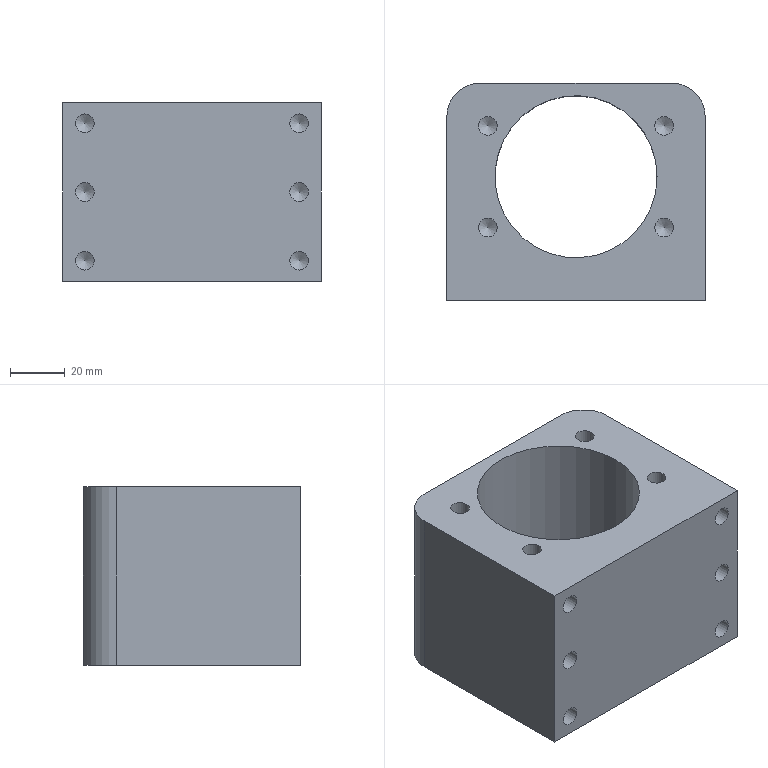Part | NX | 1 solid | 29 faces | box 94 x 79 x 65 mm | volume 292691 mm3 | cylinder 13 | cone 10 | plane 6 | commonest cylinder face diameters 6.8 x10 24 x2 59 x1
STEP:
#1=CARTESIAN_POINT('',(47.,-39.5,0.));
#2=VERTEX_POINT('',#1);
#3=CARTESIAN_POINT('',(47.,27.5,0.));
#4=VERTEX_POINT('',#3);
#5=CARTESIAN_POINT('',(47.,39.5,0.));
#6=DIRECTION('',(0.,1.,0.));
#7=VECTOR('',#6,1000.);
#8=LINE('',#5,#7);
#9=EDGE_CURVE('',#2,#4,#8,.T.);
#10=ORIENTED_EDGE('',*,*,#9,.T.);
#11=CARTESIAN_POINT('',(47.,27.5,65.));
#12=VERTEX_POINT('',#11);
#13=CARTESIAN_POINT('',(47.,27.5,65.));
#14=DIRECTION('',(0.,0.,-1.));
#15=VECTOR('',#14,1000.);
#16=LINE('',#13,#15);
#17=EDGE_CURVE('',#4,#12,#16,.F.);
#18=ORIENTED_EDGE('',*,*,#17,.T.);
#19=CARTESIAN_POINT('',(47.,-39.5,65.));
#20=VERTEX_POINT('',#19);
#21=CARTESIAN_POINT('',(47.,39.5,65.));
#22=DIRECTION('',(0.,1.,0.));
#23=VECTOR('',#22,1000.);
#24=LINE('',#21,#23);
#25=EDGE_CURVE('',#20,#12,#24,.T.);
#26=ORIENTED_EDGE('',*,*,#25,.F.);
#27=CARTESIAN_POINT('',(47.,-39.5,65.));
#28=DIRECTION('',(0.,0.,-1.));
#29=VECTOR('',#28,1000.);
#30=LINE('',#27,#29);
#31=EDGE_CURVE('',#20,#2,#30,.T.);
#32=ORIENTED_EDGE('',*,*,#31,.T.);
#33=EDGE_LOOP('',(#10,#18,#26,#32));
#34=FACE_BOUND('',#33,.T.);
#35=CARTESIAN_POINT('',(47.,39.5,65.));
#36=DIRECTION('',(-1.,0.,0.));
#37=DIRECTION('',(0.,-1.,0.));
#38=AXIS2_PLACEMENT_3D('',#35,#36,#37);
#39=PLANE('',#38);
#40=ADVANCED_FACE('',(#34),#39,.F.);
#41=CARTESIAN_POINT('',(35.,39.5,0.));
#42=VERTEX_POINT('',#41);
#43=CARTESIAN_POINT('',(-35.,39.5,0.));
#44=VERTEX_POINT('',#43);
#45=CARTESIAN_POINT('',(-47.,39.5,0.));
#46=DIRECTION('',(-1.,0.,0.));
#47=VECTOR('',#46,1000.);
#48=LINE('',#45,#47);
#49=EDGE_CURVE('',#42,#44,#48,.T.);
#50=ORIENTED_EDGE('',*,*,#49,.T.);
#51=CARTESIAN_POINT('',(-35.,39.5,65.));
#52=VERTEX_POINT('',#51);
#53=CARTESIAN_POINT('',(-35.,39.5,65.));
#54=DIRECTION('',(0.,0.,-1.));
#55=VECTOR('',#54,1000.);
#56=LINE('',#53,#55);
#57=EDGE_CURVE('',#44,#52,#56,.F.);
#58=ORIENTED_EDGE('',*,*,#57,.T.);
#59=CARTESIAN_POINT('',(35.,39.5,65.));
#60=VERTEX_POINT('',#59);
#61=CARTESIAN_POINT('',(-47.,39.5,65.));
#62=DIRECTION('',(-1.,0.,0.));
#63=VECTOR('',#62,1000.);
#64=LINE('',#61,#63);
#65=EDGE_CURVE('',#60,#52,#64,.T.);
#66=ORIENTED_EDGE('',*,*,#65,.F.);
#67=CARTESIAN_POINT('',(35.,39.5,65.));
#68=DIRECTION('',(0.,0.,-1.));
#69=VECTOR('',#68,1000.);
#70=LINE('',#67,#69);
#71=EDGE_CURVE('',#60,#42,#70,.T.);
#72=ORIENTED_EDGE('',*,*,#71,.T.);
#73=EDGE_LOOP('',(#50,#58,#66,#72));
#74=FACE_BOUND('',#73,.T.);
#75=CARTESIAN_POINT('',(-47.,39.5,65.));
#76=DIRECTION('',(0.,-1.,0.));
#77=DIRECTION('',(0.,0.,-1.));
#78=AXIS2_PLACEMENT_3D('',#75,#76,#77);
#79=PLANE('',#78);
#80=ADVANCED_FACE('',(#74),#79,.F.);
#81=CARTESIAN_POINT('',(-47.,27.5,65.));
#82=VERTEX_POINT('',#81);
#83=CARTESIAN_POINT('',(-47.,-39.5,65.));
#84=VERTEX_POINT('',#83);
#85=CARTESIAN_POINT('',(-47.,39.5,65.));
#86=DIRECTION('',(0.,-1.,0.));
#87=VECTOR('',#86,1000.);
#88=LINE('',#85,#87);
#89=EDGE_CURVE('',#82,#84,#88,.T.);
#90=ORIENTED_EDGE('',*,*,#89,.F.);
#91=CARTESIAN_POINT('',(-47.,27.5,0.));
#92=VERTEX_POINT('',#91);
#93=CARTESIAN_POINT('',(-47.,27.5,65.));
#94=DIRECTION('',(0.,0.,-1.));
#95=VECTOR('',#94,1000.);
#96=LINE('',#93,#95);
#97=EDGE_CURVE('',#82,#92,#96,.T.);
#98=ORIENTED_EDGE('',*,*,#97,.T.);
#99=CARTESIAN_POINT('',(-47.,-39.5,0.));
#100=VERTEX_POINT('',#99);
#101=CARTESIAN_POINT('',(-47.,39.5,0.));
#102=DIRECTION('',(0.,-1.,0.));
#103=VECTOR('',#102,1000.);
#104=LINE('',#101,#103);
#105=EDGE_CURVE('',#92,#100,#104,.T.);
#106=ORIENTED_EDGE('',*,*,#105,.T.);
#107=CARTESIAN_POINT('',(-47.,-39.5,65.));
#108=DIRECTION('',(0.,0.,-1.));
#109=VECTOR('',#108,1000.);
#110=LINE('',#107,#109);
#111=EDGE_CURVE('',#84,#100,#110,.T.);
#112=ORIENTED_EDGE('',*,*,#111,.F.);
#113=EDGE_LOOP('',(#90,#98,#106,#112));
#114=FACE_BOUND('',#113,.T.);
#115=CARTESIAN_POINT('',(-47.,39.5,65.));
#116=DIRECTION('',(1.,0.,0.));
#117=DIRECTION('',(0.,1.,0.));
#118=AXIS2_PLACEMENT_3D('',#115,#116,#117);
#119=PLANE('',#118);
#120=ADVANCED_FACE('',(#114),#119,.F.);
#121=CARTESIAN_POINT('',(-39.,-39.5,54.1));
#122=VERTEX_POINT('',#121);
#123=CARTESIAN_POINT('',(-39.,-39.5,57.5));
#124=DIRECTION('',(0.,-1.,0.));
#125=DIRECTION('',(0.,0.,-1.));
#126=AXIS2_PLACEMENT_3D('',#123,#124,#125);
#127=CIRCLE('',#126,3.4);
#128=EDGE_CURVE('',#122,#122,#127,.T.);
#129=ORIENTED_EDGE('',*,*,#128,.F.);
#130=EDGE_LOOP('',(#129));
#131=FACE_BOUND('',#130,.T.);
#132=CARTESIAN_POINT('',(39.,-39.5,54.1));
#133=VERTEX_POINT('',#132);
#134=CARTESIAN_POINT('',(39.,-39.5,57.5));
#135=DIRECTION('',(0.,-1.,0.));
#136=DIRECTION('',(0.,0.,-1.));
#137=AXIS2_PLACEMENT_3D('',#134,#135,#136);
#138=CIRCLE('',#137,3.4);
#139=EDGE_CURVE('',#133,#133,#138,.T.);
#140=ORIENTED_EDGE('',*,*,#139,.F.);
#141=EDGE_LOOP('',(#140));
#142=FACE_BOUND('',#141,.T.);
#143=CARTESIAN_POINT('',(39.,-39.5,29.1));
#144=VERTEX_POINT('',#143);
#145=CARTESIAN_POINT('',(39.,-39.5,32.5));
#146=DIRECTION('',(0.,-1.,0.));
#147=DIRECTION('',(0.,0.,-1.));
#148=AXIS2_PLACEMENT_3D('',#145,#146,#147);
#149=CIRCLE('',#148,3.4);
#150=EDGE_CURVE('',#144,#144,#149,.T.);
#151=ORIENTED_EDGE('',*,*,#150,.F.);
#152=EDGE_LOOP('',(#151));
#153=FACE_BOUND('',#152,.T.);
#154=CARTESIAN_POINT('',(-39.,-39.5,29.1));
#155=VERTEX_POINT('',#154);
#156=CARTESIAN_POINT('',(-39.,-39.5,32.5));
#157=DIRECTION('',(0.,-1.,0.));
#158=DIRECTION('',(0.,0.,-1.));
#159=AXIS2_PLACEMENT_3D('',#156,#157,#158);
#160=CIRCLE('',#159,3.4);
#161=EDGE_CURVE('',#155,#155,#160,.T.);
#162=ORIENTED_EDGE('',*,*,#161,.F.);
#163=EDGE_LOOP('',(#162));
#164=FACE_BOUND('',#163,.T.);
#165=CARTESIAN_POINT('',(-39.,-39.5,4.1));
#166=VERTEX_POINT('',#165);
#167=CARTESIAN_POINT('',(-39.,-39.5,7.5));
#168=DIRECTION('',(0.,-1.,0.));
#169=DIRECTION('',(0.,0.,-1.));
#170=AXIS2_PLACEMENT_3D('',#167,#168,#169);
#171=CIRCLE('',#170,3.4);
#172=EDGE_CURVE('',#166,#166,#171,.T.);
#173=ORIENTED_EDGE('',*,*,#172,.F.);
#174=EDGE_LOOP('',(#173));
#175=FACE_BOUND('',#174,.T.);
#176=CARTESIAN_POINT('',(39.,-39.5,4.1));
#177=VERTEX_POINT('',#176);
#178=CARTESIAN_POINT('',(39.,-39.5,7.5));
#179=DIRECTION('',(0.,-1.,0.));
#180=DIRECTION('',(0.,0.,-1.));
#181=AXIS2_PLACEMENT_3D('',#178,#179,#180);
#182=CIRCLE('',#181,3.4);
#183=EDGE_CURVE('',#177,#177,#182,.T.);
#184=ORIENTED_EDGE('',*,*,#183,.F.);
#185=EDGE_LOOP('',(#184));
#186=FACE_BOUND('',#185,.T.);
#187=CARTESIAN_POINT('',(-47.,-39.5,0.));
#188=DIRECTION('',(1.,0.,0.));
#189=VECTOR('',#188,1000.);
#190=LINE('',#187,#189);
#191=EDGE_CURVE('',#100,#2,#190,.T.);
#192=ORIENTED_EDGE('',*,*,#191,.T.);
#193=ORIENTED_EDGE('',*,*,#31,.F.);
#194=CARTESIAN_POINT('',(-47.,-39.5,65.));
#195=DIRECTION('',(1.,0.,0.));
#196=VECTOR('',#195,1000.);
#197=LINE('',#194,#196);
#198=EDGE_CURVE('',#84,#20,#197,.T.);
#199=ORIENTED_EDGE('',*,*,#198,.F.);
#200=ORIENTED_EDGE('',*,*,#111,.T.);
#201=EDGE_LOOP('',(#192,#193,#199,#200));
#202=FACE_BOUND('',#201,.T.);
#203=CARTESIAN_POINT('',(-47.,-39.5,65.));
#204=DIRECTION('',(0.,1.,0.));
#205=DIRECTION('',(0.,0.,1.));
#206=AXIS2_PLACEMENT_3D('',#203,#204,#205);
#207=PLANE('',#206);
#208=ADVANCED_FACE('',(#131,#142,#153,#164,#175,#186,#202),#207,.F.);
#209=CARTESIAN_POINT('',(-28.643,24.,65.));
#210=VERTEX_POINT('',#209);
#211=CARTESIAN_POINT('',(-32.043,24.,65.));
#212=DIRECTION('',(0.,0.,1.));
#213=DIRECTION('',(1.,0.,0.));
#214=AXIS2_PLACEMENT_3D('',#211,#212,#213);
#215=CIRCLE('',#214,3.4);
#216=EDGE_CURVE('',#210,#210,#215,.T.);
#217=ORIENTED_EDGE('',*,*,#216,.F.);
#218=EDGE_LOOP('',(#217));
#219=FACE_BOUND('',#218,.T.);
#220=CARTESIAN_POINT('',(-28.643,-13.,65.));
#221=VERTEX_POINT('',#220);
#222=CARTESIAN_POINT('',(-32.043,-13.,65.));
#223=DIRECTION('',(0.,0.,1.));
#224=DIRECTION('',(1.,0.,0.));
#225=AXIS2_PLACEMENT_3D('',#222,#223,#224);
#226=CIRCLE('',#225,3.4);
#227=EDGE_CURVE('',#221,#221,#226,.T.);
#228=ORIENTED_EDGE('',*,*,#227,.F.);
#229=EDGE_LOOP('',(#228));
#230=FACE_BOUND('',#229,.T.);
#231=CARTESIAN_POINT('',(35.443,-13.,65.));
#232=VERTEX_POINT('',#231);
#233=CARTESIAN_POINT('',(32.043,-13.,65.));
#234=DIRECTION('',(0.,0.,1.));
#235=DIRECTION('',(1.,0.,0.));
#236=AXIS2_PLACEMENT_3D('',#233,#234,#235);
#237=CIRCLE('',#236,3.4);
#238=EDGE_CURVE('',#232,#232,#237,.T.);
#239=ORIENTED_EDGE('',*,*,#238,.F.);
#240=EDGE_LOOP('',(#239));
#241=FACE_BOUND('',#240,.T.);
#242=CARTESIAN_POINT('',(35.443,24.,65.));
#243=VERTEX_POINT('',#242);
#244=CARTESIAN_POINT('',(32.043,24.,65.));
#245=DIRECTION('',(0.,0.,1.));
#246=DIRECTION('',(1.,0.,0.));
#247=AXIS2_PLACEMENT_3D('',#244,#245,#246);
#248=CIRCLE('',#247,3.4);
#249=EDGE_CURVE('',#243,#243,#248,.T.);
#250=ORIENTED_EDGE('',*,*,#249,.F.);
#251=EDGE_LOOP('',(#250));
#252=FACE_BOUND('',#251,.T.);
#253=CARTESIAN_POINT('',(29.5,5.5,65.));
#254=VERTEX_POINT('',#253);
#255=CARTESIAN_POINT('',(0.,5.5,65.));
#256=DIRECTION('',(0.,0.,1.));
#257=DIRECTION('',(1.,0.,0.));
#258=AXIS2_PLACEMENT_3D('',#255,#256,#257);
#259=CIRCLE('',#258,29.5);
#260=EDGE_CURVE('',#254,#254,#259,.T.);
#261=ORIENTED_EDGE('',*,*,#260,.F.);
#262=EDGE_LOOP('',(#261));
#263=FACE_BOUND('',#262,.T.);
#264=ORIENTED_EDGE('',*,*,#65,.T.);
#265=CARTESIAN_POINT('',(-35.,27.5,65.));
#266=DIRECTION('',(0.,0.,1.));
#267=DIRECTION('',(1.,0.,0.));
#268=AXIS2_PLACEMENT_3D('',#265,#266,#267);
#269=CIRCLE('',#268,12.);
#270=EDGE_CURVE('',#52,#82,#269,.T.);
#271=ORIENTED_EDGE('',*,*,#270,.T.);
#272=ORIENTED_EDGE('',*,*,#89,.T.);
#273=ORIENTED_EDGE('',*,*,#198,.T.);
#274=ORIENTED_EDGE('',*,*,#25,.T.);
#275=CARTESIAN_POINT('',(35.,27.5,65.));
#276=DIRECTION('',(0.,0.,1.));
#277=DIRECTION('',(1.,0.,0.));
#278=AXIS2_PLACEMENT_3D('',#275,#276,#277);
#279=CIRCLE('',#278,12.);
#280=EDGE_CURVE('',#12,#60,#279,.T.);
#281=ORIENTED_EDGE('',*,*,#280,.T.);
#282=EDGE_LOOP('',(#264,#271,#272,#273,#274,#281));
#283=FACE_BOUND('',#282,.T.);
#284=CARTESIAN_POINT('',(0.,0.,65.));
#285=DIRECTION('',(0.,0.,1.));
#286=DIRECTION('',(1.,0.,0.));
#287=AXIS2_PLACEMENT_3D('',#284,#285,#286);
#288=PLANE('',#287);
#289=ADVANCED_FACE('',(#219,#230,#241,#252,#263,#283),#288,.T.);
#290=CARTESIAN_POINT('',(29.5,5.5,0.));
#291=VERTEX_POINT('',#290);
#292=CARTESIAN_POINT('',(0.,5.5,0.));
#293=DIRECTION('',(0.,0.,1.));
#294=DIRECTION('',(1.,0.,0.));
#295=AXIS2_PLACEMENT_3D('',#292,#293,#294);
#296=CIRCLE('',#295,29.5);
#297=EDGE_CURVE('',#291,#291,#296,.F.);
#298=ORIENTED_EDGE('',*,*,#297,.F.);
#299=EDGE_LOOP('',(#298));
#300=FACE_BOUND('',#299,.T.);
#301=ORIENTED_EDGE('',*,*,#105,.F.);
#302=CARTESIAN_POINT('',(-35.,27.5,0.));
#303=DIRECTION('',(0.,0.,1.));
#304=DIRECTION('',(1.,0.,0.));
#305=AXIS2_PLACEMENT_3D('',#302,#303,#304);
#306=CIRCLE('',#305,12.);
#307=EDGE_CURVE('',#92,#44,#306,.F.);
#308=ORIENTED_EDGE('',*,*,#307,.T.);
#309=ORIENTED_EDGE('',*,*,#49,.F.);
#310=CARTESIAN_POINT('',(35.,27.5,0.));
#311=DIRECTION('',(0.,0.,1.));
#312=DIRECTION('',(1.,0.,0.));
#313=AXIS2_PLACEMENT_3D('',#310,#311,#312);
#314=CIRCLE('',#313,12.);
#315=EDGE_CURVE('',#42,#4,#314,.F.);
#316=ORIENTED_EDGE('',*,*,#315,.T.);
#317=ORIENTED_EDGE('',*,*,#9,.F.);
#318=ORIENTED_EDGE('',*,*,#191,.F.);
#319=EDGE_LOOP('',(#301,#308,#309,#316,#317,#318));
#320=FACE_BOUND('',#319,.T.);
#321=CARTESIAN_POINT('',(0.,0.,0.));
#322=DIRECTION('',(0.,0.,1.));
#323=DIRECTION('',(1.,0.,0.));
#324=AXIS2_PLACEMENT_3D('',#321,#322,#323);
#325=PLANE('',#324);
#326=ADVANCED_FACE('',(#300,#320),#325,.F.);
#327=ORIENTED_EDGE('',*,*,#260,.T.);
#328=EDGE_LOOP('',(#327));
#329=FACE_BOUND('',#328,.T.);
#330=ORIENTED_EDGE('',*,*,#297,.T.);
#331=EDGE_LOOP('',(#330));
#332=FACE_BOUND('',#331,.T.);
#333=CARTESIAN_POINT('',(0.,5.5,-0.001));
#334=DIRECTION('',(0.,0.,1.));
#335=DIRECTION('',(1.,0.,0.));
#336=AXIS2_PLACEMENT_3D('',#333,#334,#335);
#337=CYLINDRICAL_SURFACE('',#336,29.5);
#338=ADVANCED_FACE('',(#329,#332),#337,.F.);
#339=CARTESIAN_POINT('',(39.,-15.457,7.5));
#340=VERTEX_POINT('',#339);
#341=VERTEX_LOOP('',#340);
#342=FACE_BOUND('',#341,.T.);
#343=CARTESIAN_POINT('',(39.,-17.5,4.1));
#344=VERTEX_POINT('',#343);
#345=CARTESIAN_POINT('',(39.,-17.5,7.5));
#346=DIRECTION('',(0.,-1.,0.));
#347=DIRECTION('',(0.,0.,-1.));
#348=AXIS2_PLACEMENT_3D('',#345,#346,#347);
#349=CIRCLE('',#348,3.4);
#350=EDGE_CURVE('',#344,#344,#349,.T.);
#351=ORIENTED_EDGE('',*,*,#350,.T.);
#352=EDGE_LOOP('',(#351));
#353=FACE_BOUND('',#352,.T.);
#354=CARTESIAN_POINT('',(39.,-17.5,7.5));
#355=DIRECTION('',(0.,-1.,0.));
#356=DIRECTION('',(0.,0.,-1.));
#357=AXIS2_PLACEMENT_3D('',#354,#355,#356);
#358=CONICAL_SURFACE('',#357,3.4,1.03);
#359=ADVANCED_FACE('',(#342,#353),#358,.F.);
#360=ORIENTED_EDGE('',*,*,#350,.F.);
#361=EDGE_LOOP('',(#360));
#362=FACE_BOUND('',#361,.T.);
#363=ORIENTED_EDGE('',*,*,#183,.T.);
#364=EDGE_LOOP('',(#363));
#365=FACE_BOUND('',#364,.T.);
#366=CARTESIAN_POINT('',(39.,-39.5,7.5));
#367=DIRECTION('',(0.,-1.,0.));
#368=DIRECTION('',(0.,0.,-1.));
#369=AXIS2_PLACEMENT_3D('',#366,#367,#368);
#370=CYLINDRICAL_SURFACE('',#369,3.4);
#371=ADVANCED_FACE('',(#362,#365),#370,.F.);
#372=CARTESIAN_POINT('',(-39.,-15.457,7.5));
#373=VERTEX_POINT('',#372);
#374=VERTEX_LOOP('',#373);
#375=FACE_BOUND('',#374,.T.);
#376=CARTESIAN_POINT('',(-39.,-17.5,4.1));
#377=VERTEX_POINT('',#376);
#378=CARTESIAN_POINT('',(-39.,-17.5,7.5));
#379=DIRECTION('',(0.,-1.,0.));
#380=DIRECTION('',(0.,0.,-1.));
#381=AXIS2_PLACEMENT_3D('',#378,#379,#380);
#382=CIRCLE('',#381,3.4);
#383=EDGE_CURVE('',#377,#377,#382,.T.);
#384=ORIENTED_EDGE('',*,*,#383,.T.);
#385=EDGE_LOOP('',(#384));
#386=FACE_BOUND('',#385,.T.);
#387=CARTESIAN_POINT('',(-39.,-17.5,7.5));
#388=DIRECTION('',(0.,-1.,0.));
#389=DIRECTION('',(0.,0.,-1.));
#390=AXIS2_PLACEMENT_3D('',#387,#388,#389);
#391=CONICAL_SURFACE('',#390,3.4,1.03);
#392=ADVANCED_FACE('',(#375,#386),#391,.F.);
#393=ORIENTED_EDGE('',*,*,#383,.F.);
#394=EDGE_LOOP('',(#393));
#395=FACE_BOUND('',#394,.T.);
#396=ORIENTED_EDGE('',*,*,#172,.T.);
#397=EDGE_LOOP('',(#396));
#398=FACE_BOUND('',#397,.T.);
#399=CARTESIAN_POINT('',(-39.,-39.5,7.5));
#400=DIRECTION('',(0.,-1.,0.));
#401=DIRECTION('',(0.,0.,-1.));
#402=AXIS2_PLACEMENT_3D('',#399,#400,#401);
#403=CYLINDRICAL_SURFACE('',#402,3.4);
#404=ADVANCED_FACE('',(#395,#398),#403,.F.);
#405=CARTESIAN_POINT('',(-39.,-15.457,32.5));
#406=VERTEX_POINT('',#405);
#407=VERTEX_LOOP('',#406);
#408=FACE_BOUND('',#407,.T.);
#409=CARTESIAN_POINT('',(-39.,-17.5,29.1));
#410=VERTEX_POINT('',#409);
#411=CARTESIAN_POINT('',(-39.,-17.5,32.5));
#412=DIRECTION('',(0.,-1.,0.));
#413=DIRECTION('',(0.,0.,-1.));
#414=AXIS2_PLACEMENT_3D('',#411,#412,#413);
#415=CIRCLE('',#414,3.4);
#416=EDGE_CURVE('',#410,#410,#415,.T.);
#417=ORIENTED_EDGE('',*,*,#416,.T.);
#418=EDGE_LOOP('',(#417));
#419=FACE_BOUND('',#418,.T.);
#420=CARTESIAN_POINT('',(-39.,-17.5,32.5));
#421=DIRECTION('',(0.,-1.,0.));
#422=DIRECTION('',(0.,0.,-1.));
#423=AXIS2_PLACEMENT_3D('',#420,#421,#422);
#424=CONICAL_SURFACE('',#423,3.4,1.03);
#425=ADVANCED_FACE('',(#408,#419),#424,.F.);
#426=ORIENTED_EDGE('',*,*,#416,.F.);
#427=EDGE_LOOP('',(#426));
#428=FACE_BOUND('',#427,.T.);
#429=ORIENTED_EDGE('',*,*,#161,.T.);
#430=EDGE_LOOP('',(#429));
#431=FACE_BOUND('',#430,.T.);
#432=CARTESIAN_POINT('',(-39.,-39.5,32.5));
#433=DIRECTION('',(0.,-1.,0.));
#434=DIRECTION('',(0.,0.,-1.));
#435=AXIS2_PLACEMENT_3D('',#432,#433,#434);
#436=CYLINDRICAL_SURFACE('',#435,3.4);
#437=ADVANCED_FACE('',(#428,#431),#436,.F.);
#438=CARTESIAN_POINT('',(39.,-15.457,32.5));
#439=VERTEX_POINT('',#438);
#440=VERTEX_LOOP('',#439);
#441=FACE_BOUND('',#440,.T.);
#442=CARTESIAN_POINT('',(39.,-17.5,29.1));
#443=VERTEX_POINT('',#442);
#444=CARTESIAN_POINT('',(39.,-17.5,32.5));
#445=DIRECTION('',(0.,-1.,0.));
#446=DIRECTION('',(0.,0.,-1.));
#447=AXIS2_PLACEMENT_3D('',#444,#445,#446);
#448=CIRCLE('',#447,3.4);
#449=EDGE_CURVE('',#443,#443,#448,.T.);
#450=ORIENTED_EDGE('',*,*,#449,.T.);
#451=EDGE_LOOP('',(#450));
#452=FACE_BOUND('',#451,.T.);
#453=CARTESIAN_POINT('',(39.,-17.5,32.5));
#454=DIRECTION('',(0.,-1.,0.));
#455=DIRECTION('',(0.,0.,-1.));
#456=AXIS2_PLACEMENT_3D('',#453,#454,#455);
#457=CONICAL_SURFACE('',#456,3.4,1.03);
#458=ADVANCED_FACE('',(#441,#452),#457,.F.);
#459=ORIENTED_EDGE('',*,*,#449,.F.);
#460=EDGE_LOOP('',(#459));
#461=FACE_BOUND('',#460,.T.);
#462=ORIENTED_EDGE('',*,*,#150,.T.);
#463=EDGE_LOOP('',(#462));
#464=FACE_BOUND('',#463,.T.);
#465=CARTESIAN_POINT('',(39.,-39.5,32.5));
#466=DIRECTION('',(0.,-1.,0.));
#467=DIRECTION('',(0.,0.,-1.));
#468=AXIS2_PLACEMENT_3D('',#465,#466,#467);
#469=CYLINDRICAL_SURFACE('',#468,3.4);
#470=ADVANCED_FACE('',(#461,#464),#469,.F.);
#471=CARTESIAN_POINT('',(39.,-15.457,57.5));
#472=VERTEX_POINT('',#471);
#473=VERTEX_LOOP('',#472);
#474=FACE_BOUND('',#473,.T.);
#475=CARTESIAN_POINT('',(39.,-17.5,54.1));
#476=VERTEX_POINT('',#475);
#477=CARTESIAN_POINT('',(39.,-17.5,57.5));
#478=DIRECTION('',(0.,-1.,0.));
#479=DIRECTION('',(0.,0.,-1.));
#480=AXIS2_PLACEMENT_3D('',#477,#478,#479);
#481=CIRCLE('',#480,3.4);
#482=EDGE_CURVE('',#476,#476,#481,.T.);
#483=ORIENTED_EDGE('',*,*,#482,.T.);
#484=EDGE_LOOP('',(#483));
#485=FACE_BOUND('',#484,.T.);
#486=CARTESIAN_POINT('',(39.,-17.5,57.5));
#487=DIRECTION('',(0.,-1.,0.));
#488=DIRECTION('',(0.,0.,-1.));
#489=AXIS2_PLACEMENT_3D('',#486,#487,#488);
#490=CONICAL_SURFACE('',#489,3.4,1.03);
#491=ADVANCED_FACE('',(#474,#485),#490,.F.);
#492=ORIENTED_EDGE('',*,*,#482,.F.);
#493=EDGE_LOOP('',(#492));
#494=FACE_BOUND('',#493,.T.);
#495=ORIENTED_EDGE('',*,*,#139,.T.);
#496=EDGE_LOOP('',(#495));
#497=FACE_BOUND('',#496,.T.);
#498=CARTESIAN_POINT('',(39.,-39.5,57.5));
#499=DIRECTION('',(0.,-1.,0.));
#500=DIRECTION('',(0.,0.,-1.));
#501=AXIS2_PLACEMENT_3D('',#498,#499,#500);
#502=CYLINDRICAL_SURFACE('',#501,3.4);
#503=ADVANCED_FACE('',(#494,#497),#502,.F.);
#504=CARTESIAN_POINT('',(-39.,-15.457,57.5));
#505=VERTEX_POINT('',#504);
#506=VERTEX_LOOP('',#505);
#507=FACE_BOUND('',#506,.T.);
#508=CARTESIAN_POINT('',(-39.,-17.5,54.1));
#509=VERTEX_POINT('',#508);
#510=CARTESIAN_POINT('',(-39.,-17.5,57.5));
#511=DIRECTION('',(0.,-1.,0.));
#512=DIRECTION('',(0.,0.,-1.));
#513=AXIS2_PLACEMENT_3D('',#510,#511,#512);
#514=CIRCLE('',#513,3.4);
#515=EDGE_CURVE('',#509,#509,#514,.T.);
#516=ORIENTED_EDGE('',*,*,#515,.T.);
#517=EDGE_LOOP('',(#516));
#518=FACE_BOUND('',#517,.T.);
#519=CARTESIAN_POINT('',(-39.,-17.5,57.5));
#520=DIRECTION('',(0.,-1.,0.));
#521=DIRECTION('',(0.,0.,-1.));
#522=AXIS2_PLACEMENT_3D('',#519,#520,#521);
#523=CONICAL_SURFACE('',#522,3.4,1.03);
#524=ADVANCED_FACE('',(#507,#518),#523,.F.);
#525=ORIENTED_EDGE('',*,*,#515,.F.);
#526=EDGE_LOOP('',(#525));
#527=FACE_BOUND('',#526,.T.);
#528=ORIENTED_EDGE('',*,*,#128,.T.);
#529=EDGE_LOOP('',(#528));
#530=FACE_BOUND('',#529,.T.);
#531=CARTESIAN_POINT('',(-39.,-39.5,57.5));
#532=DIRECTION('',(0.,-1.,0.));
#533=DIRECTION('',(0.,0.,-1.));
#534=AXIS2_PLACEMENT_3D('',#531,#532,#533);
#535=CYLINDRICAL_SURFACE('',#534,3.4);
#536=ADVANCED_FACE('',(#527,#530),#535,.F.);
#537=ORIENTED_EDGE('',*,*,#270,.F.);
#538=ORIENTED_EDGE('',*,*,#57,.F.);
#539=ORIENTED_EDGE('',*,*,#307,.F.);
#540=ORIENTED_EDGE('',*,*,#97,.F.);
#541=EDGE_LOOP('',(#537,#538,#539,#540));
#542=FACE_BOUND('',#541,.T.);
#543=CARTESIAN_POINT('',(-35.,27.5,65.));
#544=DIRECTION('',(0.,0.,-1.));
#545=DIRECTION('',(-1.,0.,0.));
#546=AXIS2_PLACEMENT_3D('',#543,#544,#545);
#547=CYLINDRICAL_SURFACE('',#546,12.);
#548=ADVANCED_FACE('',(#542),#547,.T.);
#549=ORIENTED_EDGE('',*,*,#280,.F.);
#550=ORIENTED_EDGE('',*,*,#17,.F.);
#551=ORIENTED_EDGE('',*,*,#315,.F.);
#552=ORIENTED_EDGE('',*,*,#71,.F.);
#553=EDGE_LOOP('',(#549,#550,#551,#552));
#554=FACE_BOUND('',#553,.T.);
#555=CARTESIAN_POINT('',(35.,27.5,65.));
#556=DIRECTION('',(0.,0.,-1.));
#557=DIRECTION('',(-1.,0.,0.));
#558=AXIS2_PLACEMENT_3D('',#555,#556,#557);
#559=CYLINDRICAL_SURFACE('',#558,12.);
#560=ADVANCED_FACE('',(#554),#559,.T.);
#561=CARTESIAN_POINT('',(32.043,24.,40.707));
#562=VERTEX_POINT('',#561);
#563=VERTEX_LOOP('',#562);
#564=FACE_BOUND('',#563,.T.);
#565=CARTESIAN_POINT('',(35.443,24.,42.75));
#566=VERTEX_POINT('',#565);
#567=CARTESIAN_POINT('',(32.043,24.,42.75));
#568=DIRECTION('',(0.,0.,1.));
#569=DIRECTION('',(1.,0.,0.));
#570=AXIS2_PLACEMENT_3D('',#567,#568,#569);
#571=CIRCLE('',#570,3.4);
#572=EDGE_CURVE('',#566,#566,#571,.T.);
#573=ORIENTED_EDGE('',*,*,#572,.T.);
#574=EDGE_LOOP('',(#573));
#575=FACE_BOUND('',#574,.T.);
#576=CARTESIAN_POINT('',(32.043,24.,42.75));
#577=DIRECTION('',(0.,0.,1.));
#578=DIRECTION('',(1.,0.,0.));
#579=AXIS2_PLACEMENT_3D('',#576,#577,#578);
#580=CONICAL_SURFACE('',#579,3.4,1.03);
#581=ADVANCED_FACE('',(#564,#575),#580,.F.);
#582=ORIENTED_EDGE('',*,*,#572,.F.);
#583=EDGE_LOOP('',(#582));
#584=FACE_BOUND('',#583,.T.);
#585=ORIENTED_EDGE('',*,*,#249,.T.);
#586=EDGE_LOOP('',(#585));
#587=FACE_BOUND('',#586,.T.);
#588=CARTESIAN_POINT('',(32.043,24.,65.));
#589=DIRECTION('',(0.,0.,1.));
#590=DIRECTION('',(1.,0.,0.));
#591=AXIS2_PLACEMENT_3D('',#588,#589,#590);
#592=CYLINDRICAL_SURFACE('',#591,3.4);
#593=ADVANCED_FACE('',(#584,#587),#592,.F.);
#594=CARTESIAN_POINT('',(32.043,-13.,40.707));
#595=VERTEX_POINT('',#594);
#596=VERTEX_LOOP('',#595);
#597=FACE_BOUND('',#596,.T.);
#598=CARTESIAN_POINT('',(35.443,-13.,42.75));
#599=VERTEX_POINT('',#598);
#600=CARTESIAN_POINT('',(32.043,-13.,42.75));
#601=DIRECTION('',(0.,0.,1.));
#602=DIRECTION('',(1.,0.,0.));
#603=AXIS2_PLACEMENT_3D('',#600,#601,#602);
#604=CIRCLE('',#603,3.4);
#605=EDGE_CURVE('',#599,#599,#604,.T.);
#606=ORIENTED_EDGE('',*,*,#605,.T.);
#607=EDGE_LOOP('',(#606));
#608=FACE_BOUND('',#607,.T.);
#609=CARTESIAN_POINT('',(32.043,-13.,42.75));
#610=DIRECTION('',(0.,0.,1.));
#611=DIRECTION('',(1.,0.,0.));
#612=AXIS2_PLACEMENT_3D('',#609,#610,#611);
#613=CONICAL_SURFACE('',#612,3.4,1.03);
#614=ADVANCED_FACE('',(#597,#608),#613,.F.);
#615=ORIENTED_EDGE('',*,*,#605,.F.);
#616=EDGE_LOOP('',(#615));
#617=FACE_BOUND('',#616,.T.);
#618=ORIENTED_EDGE('',*,*,#238,.T.);
#619=EDGE_LOOP('',(#618));
#620=FACE_BOUND('',#619,.T.);
#621=CARTESIAN_POINT('',(32.043,-13.,65.));
#622=DIRECTION('',(0.,0.,1.));
#623=DIRECTION('',(1.,0.,0.));
#624=AXIS2_PLACEMENT_3D('',#621,#622,#623);
#625=CYLINDRICAL_SURFACE('',#624,3.4);
#626=ADVANCED_FACE('',(#617,#620),#625,.F.);
#627=CARTESIAN_POINT('',(-32.043,-13.,40.707));
#628=VERTEX_POINT('',#627);
#629=VERTEX_LOOP('',#628);
#630=FACE_BOUND('',#629,.T.);
#631=CARTESIAN_POINT('',(-28.643,-13.,42.75));
#632=VERTEX_POINT('',#631);
#633=CARTESIAN_POINT('',(-32.043,-13.,42.75));
#634=DIRECTION('',(0.,0.,1.));
#635=DIRECTION('',(1.,0.,0.));
#636=AXIS2_PLACEMENT_3D('',#633,#634,#635);
#637=CIRCLE('',#636,3.4);
#638=EDGE_CURVE('',#632,#632,#637,.T.);
#639=ORIENTED_EDGE('',*,*,#638,.T.);
#640=EDGE_LOOP('',(#639));
#641=FACE_BOUND('',#640,.T.);
#642=CARTESIAN_POINT('',(-32.043,-13.,42.75));
#643=DIRECTION('',(0.,0.,1.));
#644=DIRECTION('',(1.,0.,0.));
#645=AXIS2_PLACEMENT_3D('',#642,#643,#644);
#646=CONICAL_SURFACE('',#645,3.4,1.03);
#647=ADVANCED_FACE('',(#630,#641),#646,.F.);
#648=ORIENTED_EDGE('',*,*,#638,.F.);
#649=EDGE_LOOP('',(#648));
#650=FACE_BOUND('',#649,.T.);
#651=ORIENTED_EDGE('',*,*,#227,.T.);
#652=EDGE_LOOP('',(#651));
#653=FACE_BOUND('',#652,.T.);
#654=CARTESIAN_POINT('',(-32.043,-13.,65.));
#655=DIRECTION('',(0.,0.,1.));
#656=DIRECTION('',(1.,0.,0.));
#657=AXIS2_PLACEMENT_3D('',#654,#655,#656);
#658=CYLINDRICAL_SURFACE('',#657,3.4);
#659=ADVANCED_FACE('',(#650,#653),#658,.F.);
#660=CARTESIAN_POINT('',(-32.043,24.,40.707));
#661=VERTEX_POINT('',#660);
#662=VERTEX_LOOP('',#661);
#663=FACE_BOUND('',#662,.T.);
#664=CARTESIAN_POINT('',(-28.643,24.,42.75));
#665=VERTEX_POINT('',#664);
#666=CARTESIAN_POINT('',(-32.043,24.,42.75));
#667=DIRECTION('',(0.,0.,1.));
#668=DIRECTION('',(1.,0.,0.));
#669=AXIS2_PLACEMENT_3D('',#666,#667,#668);
#670=CIRCLE('',#669,3.4);
#671=EDGE_CURVE('',#665,#665,#670,.T.);
#672=ORIENTED_EDGE('',*,*,#671,.T.);
#673=EDGE_LOOP('',(#672));
#674=FACE_BOUND('',#673,.T.);
#675=CARTESIAN_POINT('',(-32.043,24.,42.75));
#676=DIRECTION('',(0.,0.,1.));
#677=DIRECTION('',(1.,0.,0.));
#678=AXIS2_PLACEMENT_3D('',#675,#676,#677);
#679=CONICAL_SURFACE('',#678,3.4,1.03);
#680=ADVANCED_FACE('',(#663,#674),#679,.F.);
#681=ORIENTED_EDGE('',*,*,#671,.F.);
#682=EDGE_LOOP('',(#681));
#683=FACE_BOUND('',#682,.T.);
#684=ORIENTED_EDGE('',*,*,#216,.T.);
#685=EDGE_LOOP('',(#684));
#686=FACE_BOUND('',#685,.T.);
#687=CARTESIAN_POINT('',(-32.043,24.,65.));
#688=DIRECTION('',(0.,0.,1.));
#689=DIRECTION('',(1.,0.,0.));
#690=AXIS2_PLACEMENT_3D('',#687,#688,#689);
#691=CYLINDRICAL_SURFACE('',#690,3.4);
#692=ADVANCED_FACE('',(#683,#686),#691,.F.);
#693=CLOSED_SHELL('',(#40,#80,#120,#208,#289,#326,#338,#359,#371,#392,#404,#425,#437,#458,#470,#491,#503,#524,#536,#548,#560,#581,#593,#614,#626,#647,#659,#680,#692));
#694=MANIFOLD_SOLID_BREP('',#693);
#695=(LENGTH_UNIT()NAMED_UNIT(*)SI_UNIT(.MILLI.,.METRE.));
#696=UNCERTAINTY_MEASURE_WITH_UNIT(LENGTH_MEASURE(0.00001),#695,'','');
#697=(NAMED_UNIT(*)PLANE_ANGLE_UNIT()SI_UNIT($,.RADIAN.));
#698=(NAMED_UNIT(*)SI_UNIT($,.STERADIAN.)SOLID_ANGLE_UNIT());
#699=(GEOMETRIC_REPRESENTATION_CONTEXT(3)GLOBAL_UNCERTAINTY_ASSIGNED_CONTEXT((#696))GLOBAL_UNIT_ASSIGNED_CONTEXT((#695,#697,#698))REPRESENTATION_CONTEXT('',''));
#700=ADVANCED_BREP_SHAPE_REPRESENTATION('',(#694),#699);